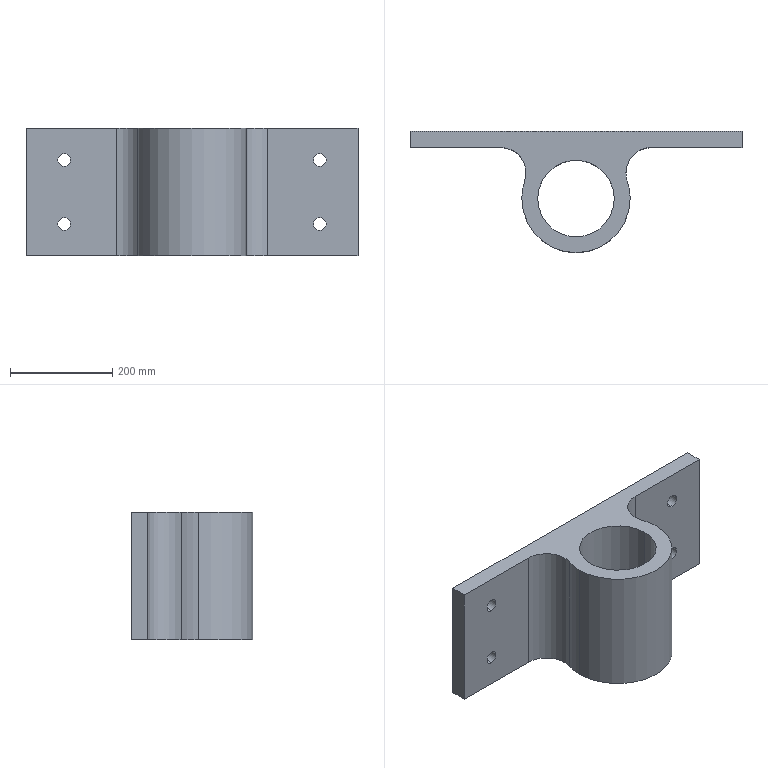Part | SolidWorks | features Extrusion 1, ICE 1 | 1 solid | 23 faces | box 650 x 238 x 250 mm | volume 10403877 mm3 | cylinder 16 | plane 7 | commonest cylinder face diameters 25 x8 100 x3 212 x3 150 x2
STEP:
#1=CARTESIAN_POINT('',(250.,100.,75.));
#2=VERTEX_POINT('',#1);
#3=CARTESIAN_POINT('',(250.,100.,50.));
#4=VERTEX_POINT('',#3);
#5=CARTESIAN_POINT('',(250.,100.,62.5));
#6=DIRECTION('',(0.,-1.,0.));
#7=DIRECTION('',(-1.,0.,0.));
#8=AXIS2_PLACEMENT_3D('',#5,#6,#7);
#9=CIRCLE('',#8,12.5);
#10=EDGE_CURVE('',#2,#4,#9,.T.);
#11=ORIENTED_EDGE('',*,*,#10,.T.);
#12=CARTESIAN_POINT('',(250.,132.,50.));
#13=VERTEX_POINT('',#12);
#14=CARTESIAN_POINT('',(250.,-106.001,50.));
#15=DIRECTION('',(0.,1.,0.));
#16=VECTOR('',#15,1000.);
#17=LINE('',#14,#16);
#18=EDGE_CURVE('',#4,#13,#17,.T.);
#19=ORIENTED_EDGE('',*,*,#18,.T.);
#20=CARTESIAN_POINT('',(250.,132.,75.));
#21=VERTEX_POINT('',#20);
#22=CARTESIAN_POINT('',(250.,132.,62.5));
#23=DIRECTION('',(0.,1.,0.));
#24=DIRECTION('',(0.,0.,1.));
#25=AXIS2_PLACEMENT_3D('',#22,#23,#24);
#26=CIRCLE('',#25,12.5);
#27=EDGE_CURVE('',#13,#21,#26,.T.);
#28=ORIENTED_EDGE('',*,*,#27,.T.);
#29=CARTESIAN_POINT('',(250.,-106.001,75.));
#30=DIRECTION('',(0.,1.,0.));
#31=VECTOR('',#30,1000.);
#32=LINE('',#29,#31);
#33=EDGE_CURVE('',#2,#21,#32,.T.);
#34=ORIENTED_EDGE('',*,*,#33,.F.);
#35=EDGE_LOOP('',(#11,#19,#28,#34));
#36=FACE_OUTER_BOUND('',#35,.T.);
#37=CARTESIAN_POINT('',(250.,-106.001,62.5));
#38=DIRECTION('',(0.,1.,0.));
#39=DIRECTION('',(0.,0.,1.));
#40=AXIS2_PLACEMENT_3D('',#37,#38,#39);
#41=CYLINDRICAL_SURFACE('',#40,12.5);
#42=ADVANCED_FACE('',(#36),#41,.F.);
#43=CARTESIAN_POINT('',(250.,100.,200.));
#44=VERTEX_POINT('',#43);
#45=CARTESIAN_POINT('',(250.,100.,175.));
#46=VERTEX_POINT('',#45);
#47=CARTESIAN_POINT('',(250.,100.,187.5));
#48=DIRECTION('',(0.,-1.,0.));
#49=DIRECTION('',(-1.,0.,0.));
#50=AXIS2_PLACEMENT_3D('',#47,#48,#49);
#51=CIRCLE('',#50,12.5);
#52=EDGE_CURVE('',#44,#46,#51,.T.);
#53=ORIENTED_EDGE('',*,*,#52,.T.);
#54=CARTESIAN_POINT('',(250.,132.,175.));
#55=VERTEX_POINT('',#54);
#56=CARTESIAN_POINT('',(250.,-106.001,175.));
#57=DIRECTION('',(0.,1.,0.));
#58=VECTOR('',#57,1000.);
#59=LINE('',#56,#58);
#60=EDGE_CURVE('',#46,#55,#59,.T.);
#61=ORIENTED_EDGE('',*,*,#60,.T.);
#62=CARTESIAN_POINT('',(250.,132.,200.));
#63=VERTEX_POINT('',#62);
#64=CARTESIAN_POINT('',(250.,132.,187.5));
#65=DIRECTION('',(0.,1.,0.));
#66=DIRECTION('',(0.,0.,1.));
#67=AXIS2_PLACEMENT_3D('',#64,#65,#66);
#68=CIRCLE('',#67,12.5);
#69=EDGE_CURVE('',#55,#63,#68,.T.);
#70=ORIENTED_EDGE('',*,*,#69,.T.);
#71=CARTESIAN_POINT('',(250.,-106.001,200.));
#72=DIRECTION('',(0.,1.,0.));
#73=VECTOR('',#72,1000.);
#74=LINE('',#71,#73);
#75=EDGE_CURVE('',#44,#63,#74,.T.);
#76=ORIENTED_EDGE('',*,*,#75,.F.);
#77=EDGE_LOOP('',(#53,#61,#70,#76));
#78=FACE_OUTER_BOUND('',#77,.T.);
#79=CARTESIAN_POINT('',(250.,-106.001,187.5));
#80=DIRECTION('',(0.,1.,0.));
#81=DIRECTION('',(0.,0.,1.));
#82=AXIS2_PLACEMENT_3D('',#79,#80,#81);
#83=CYLINDRICAL_SURFACE('',#82,12.5);
#84=ADVANCED_FACE('',(#78),#83,.F.);
#85=CARTESIAN_POINT('',(-250.,100.,200.));
#86=VERTEX_POINT('',#85);
#87=CARTESIAN_POINT('',(-250.,100.,175.));
#88=VERTEX_POINT('',#87);
#89=CARTESIAN_POINT('',(-250.,100.,187.5));
#90=DIRECTION('',(0.,-1.,0.));
#91=DIRECTION('',(-1.,0.,0.));
#92=AXIS2_PLACEMENT_3D('',#89,#90,#91);
#93=CIRCLE('',#92,12.5);
#94=EDGE_CURVE('',#86,#88,#93,.T.);
#95=ORIENTED_EDGE('',*,*,#94,.T.);
#96=CARTESIAN_POINT('',(-250.,132.,175.));
#97=VERTEX_POINT('',#96);
#98=CARTESIAN_POINT('',(-250.,-106.001,175.));
#99=DIRECTION('',(0.,1.,0.));
#100=VECTOR('',#99,1000.);
#101=LINE('',#98,#100);
#102=EDGE_CURVE('',#88,#97,#101,.T.);
#103=ORIENTED_EDGE('',*,*,#102,.T.);
#104=CARTESIAN_POINT('',(-250.,132.,200.));
#105=VERTEX_POINT('',#104);
#106=CARTESIAN_POINT('',(-250.,132.,187.5));
#107=DIRECTION('',(0.,1.,0.));
#108=DIRECTION('',(0.,0.,1.));
#109=AXIS2_PLACEMENT_3D('',#106,#107,#108);
#110=CIRCLE('',#109,12.5);
#111=EDGE_CURVE('',#97,#105,#110,.T.);
#112=ORIENTED_EDGE('',*,*,#111,.T.);
#113=CARTESIAN_POINT('',(-250.,-106.001,200.));
#114=DIRECTION('',(0.,1.,0.));
#115=VECTOR('',#114,1000.);
#116=LINE('',#113,#115);
#117=EDGE_CURVE('',#86,#105,#116,.T.);
#118=ORIENTED_EDGE('',*,*,#117,.F.);
#119=EDGE_LOOP('',(#95,#103,#112,#118));
#120=FACE_OUTER_BOUND('',#119,.T.);
#121=CARTESIAN_POINT('',(-250.,-106.001,187.5));
#122=DIRECTION('',(0.,1.,0.));
#123=DIRECTION('',(0.,0.,1.));
#124=AXIS2_PLACEMENT_3D('',#121,#122,#123);
#125=CYLINDRICAL_SURFACE('',#124,12.5);
#126=ADVANCED_FACE('',(#120),#125,.F.);
#127=CARTESIAN_POINT('',(-250.,100.,75.));
#128=VERTEX_POINT('',#127);
#129=CARTESIAN_POINT('',(-250.,100.,50.));
#130=VERTEX_POINT('',#129);
#131=CARTESIAN_POINT('',(-250.,100.,62.5));
#132=DIRECTION('',(0.,-1.,0.));
#133=DIRECTION('',(-1.,0.,0.));
#134=AXIS2_PLACEMENT_3D('',#131,#132,#133);
#135=CIRCLE('',#134,12.5);
#136=EDGE_CURVE('',#128,#130,#135,.T.);
#137=ORIENTED_EDGE('',*,*,#136,.T.);
#138=CARTESIAN_POINT('',(-250.,132.,50.));
#139=VERTEX_POINT('',#138);
#140=CARTESIAN_POINT('',(-250.,-106.001,50.));
#141=DIRECTION('',(0.,1.,0.));
#142=VECTOR('',#141,1000.);
#143=LINE('',#140,#142);
#144=EDGE_CURVE('',#130,#139,#143,.T.);
#145=ORIENTED_EDGE('',*,*,#144,.T.);
#146=CARTESIAN_POINT('',(-250.,132.,75.));
#147=VERTEX_POINT('',#146);
#148=CARTESIAN_POINT('',(-250.,132.,62.5));
#149=DIRECTION('',(0.,1.,0.));
#150=DIRECTION('',(0.,0.,1.));
#151=AXIS2_PLACEMENT_3D('',#148,#149,#150);
#152=CIRCLE('',#151,12.5);
#153=EDGE_CURVE('',#139,#147,#152,.T.);
#154=ORIENTED_EDGE('',*,*,#153,.T.);
#155=CARTESIAN_POINT('',(-250.,-106.001,75.));
#156=DIRECTION('',(0.,1.,0.));
#157=VECTOR('',#156,1000.);
#158=LINE('',#155,#157);
#159=EDGE_CURVE('',#128,#147,#158,.T.);
#160=ORIENTED_EDGE('',*,*,#159,.F.);
#161=EDGE_LOOP('',(#137,#145,#154,#160));
#162=FACE_OUTER_BOUND('',#161,.T.);
#163=CARTESIAN_POINT('',(-250.,-106.001,62.5));
#164=DIRECTION('',(0.,1.,0.));
#165=DIRECTION('',(0.,0.,1.));
#166=AXIS2_PLACEMENT_3D('',#163,#164,#165);
#167=CYLINDRICAL_SURFACE('',#166,12.5);
#168=ADVANCED_FACE('',(#162),#167,.F.);
#169=CARTESIAN_POINT('',(-75.,0.,250.));
#170=VERTEX_POINT('',#169);
#171=CARTESIAN_POINT('',(75.,0.,250.));
#172=VERTEX_POINT('',#171);
#173=CARTESIAN_POINT('',(0.,0.,250.));
#174=DIRECTION('',(0.,0.,1.));
#175=DIRECTION('',(1.,0.,0.));
#176=AXIS2_PLACEMENT_3D('',#173,#174,#175);
#177=CIRCLE('',#176,75.);
#178=EDGE_CURVE('',#170,#172,#177,.T.);
#179=ORIENTED_EDGE('',*,*,#178,.T.);
#180=CARTESIAN_POINT('',(75.,0.,0.));
#181=VERTEX_POINT('',#180);
#182=CARTESIAN_POINT('',(75.,0.,250.));
#183=DIRECTION('',(0.,0.,-1.));
#184=VECTOR('',#183,1000.);
#185=LINE('',#182,#184);
#186=EDGE_CURVE('',#172,#181,#185,.T.);
#187=ORIENTED_EDGE('',*,*,#186,.T.);
#188=CARTESIAN_POINT('',(-75.,0.,0.));
#189=VERTEX_POINT('',#188);
#190=CARTESIAN_POINT('',(0.,0.,0.));
#191=DIRECTION('',(0.,0.,1.));
#192=DIRECTION('',(1.,0.,0.));
#193=AXIS2_PLACEMENT_3D('',#190,#191,#192);
#194=CIRCLE('',#193,75.);
#195=EDGE_CURVE('',#189,#181,#194,.T.);
#196=ORIENTED_EDGE('',*,*,#195,.F.);
#197=CARTESIAN_POINT('',(-75.,0.,250.));
#198=DIRECTION('',(0.,0.,-1.));
#199=VECTOR('',#198,1000.);
#200=LINE('',#197,#199);
#201=EDGE_CURVE('',#170,#189,#200,.T.);
#202=ORIENTED_EDGE('',*,*,#201,.F.);
#203=EDGE_LOOP('',(#179,#187,#196,#202));
#204=FACE_OUTER_BOUND('',#203,.T.);
#205=CARTESIAN_POINT('',(0.,0.,250.));
#206=DIRECTION('',(0.,0.,-1.));
#207=DIRECTION('',(-1.,0.,0.));
#208=AXIS2_PLACEMENT_3D('',#205,#206,#207);
#209=CYLINDRICAL_SURFACE('',#208,75.);
#210=ADVANCED_FACE('',(#204),#209,.F.);
#211=CARTESIAN_POINT('',(97.77,50.,250.));
#212=VERTEX_POINT('',#211);
#213=CARTESIAN_POINT('',(147.77,100.,250.));
#214=VERTEX_POINT('',#213);
#215=CARTESIAN_POINT('',(147.77,50.,250.));
#216=DIRECTION('',(0.,0.,-1.));
#217=DIRECTION('',(-1.,0.,0.));
#218=AXIS2_PLACEMENT_3D('',#215,#216,#217);
#219=CIRCLE('',#218,50.);
#220=EDGE_CURVE('',#212,#214,#219,.T.);
#221=ORIENTED_EDGE('',*,*,#220,.F.);
#222=CARTESIAN_POINT('',(97.77,50.,0.));
#223=VERTEX_POINT('',#222);
#224=CARTESIAN_POINT('',(97.77,50.,250.));
#225=DIRECTION('',(0.,0.,-1.));
#226=VECTOR('',#225,1000.);
#227=LINE('',#224,#226);
#228=EDGE_CURVE('',#212,#223,#227,.T.);
#229=ORIENTED_EDGE('',*,*,#228,.T.);
#230=CARTESIAN_POINT('',(147.77,100.,0.));
#231=VERTEX_POINT('',#230);
#232=CARTESIAN_POINT('',(147.77,50.,0.));
#233=DIRECTION('',(0.,0.,-1.));
#234=DIRECTION('',(-1.,0.,0.));
#235=AXIS2_PLACEMENT_3D('',#232,#233,#234);
#236=CIRCLE('',#235,50.);
#237=EDGE_CURVE('',#223,#231,#236,.T.);
#238=ORIENTED_EDGE('',*,*,#237,.T.);
#239=CARTESIAN_POINT('',(147.77,100.,250.));
#240=DIRECTION('',(0.,0.,-1.));
#241=VECTOR('',#240,1000.);
#242=LINE('',#239,#241);
#243=EDGE_CURVE('',#214,#231,#242,.T.);
#244=ORIENTED_EDGE('',*,*,#243,.F.);
#245=EDGE_LOOP('',(#221,#229,#238,#244));
#246=FACE_OUTER_BOUND('',#245,.T.);
#247=CARTESIAN_POINT('',(147.77,50.,250.));
#248=DIRECTION('',(0.,0.,-1.));
#249=DIRECTION('',(-1.,0.,0.));
#250=AXIS2_PLACEMENT_3D('',#247,#248,#249);
#251=CYLINDRICAL_SURFACE('',#250,50.);
#252=ADVANCED_FACE('',(#246),#251,.F.);
#253=CARTESIAN_POINT('',(106.,0.,250.));
#254=VERTEX_POINT('',#253);
#255=CARTESIAN_POINT('',(100.408,33.974,250.));
#256=VERTEX_POINT('',#255);
#257=CARTESIAN_POINT('',(0.,0.,250.));
#258=DIRECTION('',(0.,0.,1.));
#259=DIRECTION('',(1.,0.,0.));
#260=AXIS2_PLACEMENT_3D('',#257,#258,#259);
#261=CIRCLE('',#260,106.);
#262=EDGE_CURVE('',#254,#256,#261,.T.);
#263=ORIENTED_EDGE('',*,*,#262,.F.);
#264=CARTESIAN_POINT('',(106.,0.,0.));
#265=VERTEX_POINT('',#264);
#266=CARTESIAN_POINT('',(106.,0.,250.));
#267=DIRECTION('',(0.,0.,-1.));
#268=VECTOR('',#267,1000.);
#269=LINE('',#266,#268);
#270=EDGE_CURVE('',#254,#265,#269,.T.);
#271=ORIENTED_EDGE('',*,*,#270,.T.);
#272=CARTESIAN_POINT('',(100.408,33.974,0.));
#273=VERTEX_POINT('',#272);
#274=CARTESIAN_POINT('',(0.,0.,0.));
#275=DIRECTION('',(0.,0.,1.));
#276=DIRECTION('',(1.,0.,0.));
#277=AXIS2_PLACEMENT_3D('',#274,#275,#276);
#278=CIRCLE('',#277,106.);
#279=EDGE_CURVE('',#265,#273,#278,.T.);
#280=ORIENTED_EDGE('',*,*,#279,.T.);
#281=CARTESIAN_POINT('',(100.408,33.974,250.));
#282=DIRECTION('',(0.,0.,-1.));
#283=VECTOR('',#282,1000.);
#284=LINE('',#281,#283);
#285=EDGE_CURVE('',#256,#273,#284,.T.);
#286=ORIENTED_EDGE('',*,*,#285,.F.);
#287=EDGE_LOOP('',(#263,#271,#280,#286));
#288=FACE_OUTER_BOUND('',#287,.T.);
#289=CARTESIAN_POINT('',(0.,0.,250.));
#290=DIRECTION('',(0.,0.,-1.));
#291=DIRECTION('',(-1.,0.,0.));
#292=AXIS2_PLACEMENT_3D('',#289,#290,#291);
#293=CYLINDRICAL_SURFACE('',#292,106.);
#294=ADVANCED_FACE('',(#288),#293,.T.);
#295=ORIENTED_EDGE('',*,*,#270,.F.);
#296=CARTESIAN_POINT('',(-106.,0.,250.));
#297=VERTEX_POINT('',#296);
#298=CARTESIAN_POINT('',(0.,0.,250.));
#299=DIRECTION('',(0.,0.,1.));
#300=DIRECTION('',(1.,0.,0.));
#301=AXIS2_PLACEMENT_3D('',#298,#299,#300);
#302=CIRCLE('',#301,106.);
#303=EDGE_CURVE('',#297,#254,#302,.T.);
#304=ORIENTED_EDGE('',*,*,#303,.F.);
#305=CARTESIAN_POINT('',(-106.,0.,0.));
#306=VERTEX_POINT('',#305);
#307=CARTESIAN_POINT('',(-106.,0.,250.));
#308=DIRECTION('',(0.,0.,-1.));
#309=VECTOR('',#308,1000.);
#310=LINE('',#307,#309);
#311=EDGE_CURVE('',#297,#306,#310,.T.);
#312=ORIENTED_EDGE('',*,*,#311,.T.);
#313=CARTESIAN_POINT('',(0.,0.,0.));
#314=DIRECTION('',(0.,0.,1.));
#315=DIRECTION('',(1.,0.,0.));
#316=AXIS2_PLACEMENT_3D('',#313,#314,#315);
#317=CIRCLE('',#316,106.);
#318=EDGE_CURVE('',#306,#265,#317,.T.);
#319=ORIENTED_EDGE('',*,*,#318,.T.);
#320=EDGE_LOOP('',(#295,#304,#312,#319));
#321=FACE_OUTER_BOUND('',#320,.T.);
#322=CARTESIAN_POINT('',(0.,0.,250.));
#323=DIRECTION('',(0.,0.,-1.));
#324=DIRECTION('',(-1.,0.,0.));
#325=AXIS2_PLACEMENT_3D('',#322,#323,#324);
#326=CYLINDRICAL_SURFACE('',#325,106.);
#327=ADVANCED_FACE('',(#321),#326,.T.);
#328=CARTESIAN_POINT('',(325.,100.,250.));
#329=VERTEX_POINT('',#328);
#330=CARTESIAN_POINT('',(325.,132.,250.));
#331=VERTEX_POINT('',#330);
#332=CARTESIAN_POINT('',(325.,132.,250.));
#333=DIRECTION('',(0.,1.,0.));
#334=VECTOR('',#333,1000.);
#335=LINE('',#332,#334);
#336=EDGE_CURVE('',#329,#331,#335,.T.);
#337=ORIENTED_EDGE('',*,*,#336,.T.);
#338=CARTESIAN_POINT('',(-325.,132.,250.));
#339=VERTEX_POINT('',#338);
#340=CARTESIAN_POINT('',(325.,132.,250.));
#341=DIRECTION('',(-1.,0.,0.));
#342=VECTOR('',#341,1000.);
#343=LINE('',#340,#342);
#344=EDGE_CURVE('',#331,#339,#343,.T.);
#345=ORIENTED_EDGE('',*,*,#344,.T.);
#346=CARTESIAN_POINT('',(-325.,100.,250.));
#347=VERTEX_POINT('',#346);
#348=CARTESIAN_POINT('',(-325.,132.,250.));
#349=DIRECTION('',(0.,-1.,0.));
#350=VECTOR('',#349,1000.);
#351=LINE('',#348,#350);
#352=EDGE_CURVE('',#339,#347,#351,.T.);
#353=ORIENTED_EDGE('',*,*,#352,.T.);
#354=CARTESIAN_POINT('',(-147.77,100.,250.));
#355=VERTEX_POINT('',#354);
#356=CARTESIAN_POINT('',(-325.,100.,250.));
#357=DIRECTION('',(1.,0.,0.));
#358=VECTOR('',#357,1000.);
#359=LINE('',#356,#358);
#360=EDGE_CURVE('',#347,#355,#359,.T.);
#361=ORIENTED_EDGE('',*,*,#360,.T.);
#362=CARTESIAN_POINT('',(-100.408,33.974,250.));
#363=VERTEX_POINT('',#362);
#364=CARTESIAN_POINT('',(-147.77,50.,250.));
#365=DIRECTION('',(0.,0.,-1.));
#366=DIRECTION('',(1.,0.,0.));
#367=AXIS2_PLACEMENT_3D('',#364,#365,#366);
#368=CIRCLE('',#367,50.);
#369=EDGE_CURVE('',#355,#363,#368,.T.);
#370=ORIENTED_EDGE('',*,*,#369,.T.);
#371=CARTESIAN_POINT('',(0.,0.,250.));
#372=DIRECTION('',(0.,0.,1.));
#373=DIRECTION('',(1.,0.,0.));
#374=AXIS2_PLACEMENT_3D('',#371,#372,#373);
#375=CIRCLE('',#374,106.);
#376=EDGE_CURVE('',#363,#297,#375,.T.);
#377=ORIENTED_EDGE('',*,*,#376,.T.);
#378=ORIENTED_EDGE('',*,*,#303,.T.);
#379=ORIENTED_EDGE('',*,*,#262,.T.);
#380=CARTESIAN_POINT('',(147.77,50.,250.));
#381=DIRECTION('',(0.,0.,-1.));
#382=DIRECTION('',(-1.,0.,0.));
#383=AXIS2_PLACEMENT_3D('',#380,#381,#382);
#384=CIRCLE('',#383,50.);
#385=EDGE_CURVE('',#256,#212,#384,.T.);
#386=ORIENTED_EDGE('',*,*,#385,.T.);
#387=ORIENTED_EDGE('',*,*,#220,.T.);
#388=CARTESIAN_POINT('',(325.,100.,250.));
#389=DIRECTION('',(1.,0.,0.));
#390=VECTOR('',#389,1000.);
#391=LINE('',#388,#390);
#392=EDGE_CURVE('',#214,#329,#391,.T.);
#393=ORIENTED_EDGE('',*,*,#392,.T.);
#394=EDGE_LOOP('',(#337,#345,#353,#361,#370,#377,#378,#379,#386,#387,#393));
#395=FACE_OUTER_BOUND('',#394,.T.);
#396=ORIENTED_EDGE('',*,*,#178,.F.);
#397=CARTESIAN_POINT('',(0.,0.,250.));
#398=DIRECTION('',(0.,0.,1.));
#399=DIRECTION('',(1.,0.,0.));
#400=AXIS2_PLACEMENT_3D('',#397,#398,#399);
#401=CIRCLE('',#400,75.);
#402=EDGE_CURVE('',#172,#170,#401,.T.);
#403=ORIENTED_EDGE('',*,*,#402,.F.);
#404=EDGE_LOOP('',(#396,#403));
#405=FACE_BOUND('',#404,.T.);
#406=CARTESIAN_POINT('',(147.77,50.,250.));
#407=DIRECTION('',(0.,0.,-1.));
#408=DIRECTION('',(-1.,0.,0.));
#409=AXIS2_PLACEMENT_3D('',#406,#407,#408);
#410=PLANE('',#409);
#411=ADVANCED_FACE('',(#395,#405),#410,.F.);
#412=CARTESIAN_POINT('',(325.,100.,0.));
#413=VERTEX_POINT('',#412);
#414=CARTESIAN_POINT('',(325.,132.,0.));
#415=VERTEX_POINT('',#414);
#416=CARTESIAN_POINT('',(325.,132.,0.));
#417=DIRECTION('',(0.,1.,0.));
#418=VECTOR('',#417,1000.);
#419=LINE('',#416,#418);
#420=EDGE_CURVE('',#413,#415,#419,.T.);
#421=ORIENTED_EDGE('',*,*,#420,.F.);
#422=CARTESIAN_POINT('',(325.,100.,0.));
#423=DIRECTION('',(1.,0.,0.));
#424=VECTOR('',#423,1000.);
#425=LINE('',#422,#424);
#426=EDGE_CURVE('',#231,#413,#425,.T.);
#427=ORIENTED_EDGE('',*,*,#426,.F.);
#428=ORIENTED_EDGE('',*,*,#237,.F.);
#429=CARTESIAN_POINT('',(147.77,50.,0.));
#430=DIRECTION('',(0.,0.,-1.));
#431=DIRECTION('',(-1.,0.,0.));
#432=AXIS2_PLACEMENT_3D('',#429,#430,#431);
#433=CIRCLE('',#432,50.);
#434=EDGE_CURVE('',#273,#223,#433,.T.);
#435=ORIENTED_EDGE('',*,*,#434,.F.);
#436=ORIENTED_EDGE('',*,*,#279,.F.);
#437=ORIENTED_EDGE('',*,*,#318,.F.);
#438=CARTESIAN_POINT('',(-100.408,33.974,0.));
#439=VERTEX_POINT('',#438);
#440=CARTESIAN_POINT('',(0.,0.,0.));
#441=DIRECTION('',(0.,0.,1.));
#442=DIRECTION('',(1.,0.,0.));
#443=AXIS2_PLACEMENT_3D('',#440,#441,#442);
#444=CIRCLE('',#443,106.);
#445=EDGE_CURVE('',#439,#306,#444,.T.);
#446=ORIENTED_EDGE('',*,*,#445,.F.);
#447=CARTESIAN_POINT('',(-147.77,100.,0.));
#448=VERTEX_POINT('',#447);
#449=CARTESIAN_POINT('',(-147.77,50.,0.));
#450=DIRECTION('',(0.,0.,-1.));
#451=DIRECTION('',(1.,0.,0.));
#452=AXIS2_PLACEMENT_3D('',#449,#450,#451);
#453=CIRCLE('',#452,50.);
#454=EDGE_CURVE('',#448,#439,#453,.T.);
#455=ORIENTED_EDGE('',*,*,#454,.F.);
#456=CARTESIAN_POINT('',(-325.,100.,0.));
#457=VERTEX_POINT('',#456);
#458=CARTESIAN_POINT('',(-325.,100.,0.));
#459=DIRECTION('',(1.,0.,0.));
#460=VECTOR('',#459,1000.);
#461=LINE('',#458,#460);
#462=EDGE_CURVE('',#457,#448,#461,.T.);
#463=ORIENTED_EDGE('',*,*,#462,.F.);
#464=CARTESIAN_POINT('',(-325.,132.,0.));
#465=VERTEX_POINT('',#464);
#466=CARTESIAN_POINT('',(-325.,132.,0.));
#467=DIRECTION('',(0.,-1.,0.));
#468=VECTOR('',#467,1000.);
#469=LINE('',#466,#468);
#470=EDGE_CURVE('',#465,#457,#469,.T.);
#471=ORIENTED_EDGE('',*,*,#470,.F.);
#472=CARTESIAN_POINT('',(325.,132.,0.));
#473=DIRECTION('',(-1.,0.,0.));
#474=VECTOR('',#473,1000.);
#475=LINE('',#472,#474);
#476=EDGE_CURVE('',#415,#465,#475,.T.);
#477=ORIENTED_EDGE('',*,*,#476,.F.);
#478=EDGE_LOOP('',(#421,#427,#428,#435,#436,#437,#446,#455,#463,#471,#477));
#479=FACE_OUTER_BOUND('',#478,.T.);
#480=ORIENTED_EDGE('',*,*,#195,.T.);
#481=CARTESIAN_POINT('',(0.,0.,0.));
#482=DIRECTION('',(0.,0.,1.));
#483=DIRECTION('',(1.,0.,0.));
#484=AXIS2_PLACEMENT_3D('',#481,#482,#483);
#485=CIRCLE('',#484,75.);
#486=EDGE_CURVE('',#181,#189,#485,.T.);
#487=ORIENTED_EDGE('',*,*,#486,.T.);
#488=EDGE_LOOP('',(#480,#487));
#489=FACE_BOUND('',#488,.T.);
#490=CARTESIAN_POINT('',(147.77,50.,0.));
#491=DIRECTION('',(0.,0.,-1.));
#492=DIRECTION('',(-1.,0.,0.));
#493=AXIS2_PLACEMENT_3D('',#490,#491,#492);
#494=PLANE('',#493);
#495=ADVANCED_FACE('',(#479,#489),#494,.T.);
#496=ORIENTED_EDGE('',*,*,#420,.T.);
#497=CARTESIAN_POINT('',(325.,132.,250.));
#498=DIRECTION('',(0.,0.,-1.));
#499=VECTOR('',#498,1000.);
#500=LINE('',#497,#499);
#501=EDGE_CURVE('',#331,#415,#500,.T.);
#502=ORIENTED_EDGE('',*,*,#501,.F.);
#503=ORIENTED_EDGE('',*,*,#336,.F.);
#504=CARTESIAN_POINT('',(325.,100.,250.));
#505=DIRECTION('',(0.,0.,-1.));
#506=VECTOR('',#505,1000.);
#507=LINE('',#504,#506);
#508=EDGE_CURVE('',#329,#413,#507,.T.);
#509=ORIENTED_EDGE('',*,*,#508,.T.);
#510=EDGE_LOOP('',(#496,#502,#503,#509));
#511=FACE_OUTER_BOUND('',#510,.T.);
#512=CARTESIAN_POINT('',(325.,132.,250.));
#513=DIRECTION('',(-1.,0.,0.));
#514=DIRECTION('',(0.,-1.,0.));
#515=AXIS2_PLACEMENT_3D('',#512,#513,#514);
#516=PLANE('',#515);
#517=ADVANCED_FACE('',(#511),#516,.F.);
#518=CARTESIAN_POINT('',(250.,132.,62.5));
#519=DIRECTION('',(0.,1.,0.));
#520=DIRECTION('',(0.,0.,1.));
#521=AXIS2_PLACEMENT_3D('',#518,#519,#520);
#522=CIRCLE('',#521,12.5);
#523=EDGE_CURVE('',#21,#13,#522,.T.);
#524=ORIENTED_EDGE('',*,*,#523,.F.);
#525=ORIENTED_EDGE('',*,*,#27,.F.);
#526=EDGE_LOOP('',(#524,#525));
#527=FACE_BOUND('',#526,.T.);
#528=CARTESIAN_POINT('',(250.,132.,187.5));
#529=DIRECTION('',(0.,1.,0.));
#530=DIRECTION('',(0.,0.,1.));
#531=AXIS2_PLACEMENT_3D('',#528,#529,#530);
#532=CIRCLE('',#531,12.5);
#533=EDGE_CURVE('',#63,#55,#532,.T.);
#534=ORIENTED_EDGE('',*,*,#533,.F.);
#535=ORIENTED_EDGE('',*,*,#69,.F.);
#536=EDGE_LOOP('',(#534,#535));
#537=FACE_BOUND('',#536,.T.);
#538=CARTESIAN_POINT('',(-250.,132.,187.5));
#539=DIRECTION('',(0.,1.,0.));
#540=DIRECTION('',(0.,0.,1.));
#541=AXIS2_PLACEMENT_3D('',#538,#539,#540);
#542=CIRCLE('',#541,12.5);
#543=EDGE_CURVE('',#105,#97,#542,.T.);
#544=ORIENTED_EDGE('',*,*,#543,.F.);
#545=ORIENTED_EDGE('',*,*,#111,.F.);
#546=EDGE_LOOP('',(#544,#545));
#547=FACE_BOUND('',#546,.T.);
#548=CARTESIAN_POINT('',(-250.,132.,62.5));
#549=DIRECTION('',(0.,1.,0.));
#550=DIRECTION('',(0.,0.,1.));
#551=AXIS2_PLACEMENT_3D('',#548,#549,#550);
#552=CIRCLE('',#551,12.5);
#553=EDGE_CURVE('',#147,#139,#552,.T.);
#554=ORIENTED_EDGE('',*,*,#553,.F.);
#555=ORIENTED_EDGE('',*,*,#153,.F.);
#556=EDGE_LOOP('',(#554,#555));
#557=FACE_BOUND('',#556,.T.);
#558=ORIENTED_EDGE('',*,*,#476,.T.);
#559=CARTESIAN_POINT('',(-325.,132.,250.));
#560=DIRECTION('',(0.,0.,-1.));
#561=VECTOR('',#560,1000.);
#562=LINE('',#559,#561);
#563=EDGE_CURVE('',#339,#465,#562,.T.);
#564=ORIENTED_EDGE('',*,*,#563,.F.);
#565=ORIENTED_EDGE('',*,*,#344,.F.);
#566=ORIENTED_EDGE('',*,*,#501,.T.);
#567=EDGE_LOOP('',(#558,#564,#565,#566));
#568=FACE_OUTER_BOUND('',#567,.T.);
#569=CARTESIAN_POINT('',(325.,132.,250.));
#570=DIRECTION('',(0.,-1.,0.));
#571=DIRECTION('',(0.,0.,-1.));
#572=AXIS2_PLACEMENT_3D('',#569,#570,#571);
#573=PLANE('',#572);
#574=ADVANCED_FACE('',(#527,#537,#547,#557,#568),#573,.F.);
#575=ORIENTED_EDGE('',*,*,#470,.T.);
#576=CARTESIAN_POINT('',(-325.,100.,250.));
#577=DIRECTION('',(0.,0.,-1.));
#578=VECTOR('',#577,1000.);
#579=LINE('',#576,#578);
#580=EDGE_CURVE('',#347,#457,#579,.T.);
#581=ORIENTED_EDGE('',*,*,#580,.F.);
#582=ORIENTED_EDGE('',*,*,#352,.F.);
#583=ORIENTED_EDGE('',*,*,#563,.T.);
#584=EDGE_LOOP('',(#575,#581,#582,#583));
#585=FACE_OUTER_BOUND('',#584,.T.);
#586=CARTESIAN_POINT('',(-325.,132.,250.));
#587=DIRECTION('',(1.,0.,0.));
#588=DIRECTION('',(0.,1.,0.));
#589=AXIS2_PLACEMENT_3D('',#586,#587,#588);
#590=PLANE('',#589);
#591=ADVANCED_FACE('',(#585),#590,.F.);
#592=ORIENTED_EDGE('',*,*,#94,.F.);
#593=CARTESIAN_POINT('',(-250.,100.,187.5));
#594=DIRECTION('',(0.,-1.,0.));
#595=DIRECTION('',(-1.,0.,0.));
#596=AXIS2_PLACEMENT_3D('',#593,#594,#595);
#597=CIRCLE('',#596,12.5);
#598=EDGE_CURVE('',#88,#86,#597,.T.);
#599=ORIENTED_EDGE('',*,*,#598,.F.);
#600=EDGE_LOOP('',(#592,#599));
#601=FACE_BOUND('',#600,.T.);
#602=ORIENTED_EDGE('',*,*,#136,.F.);
#603=CARTESIAN_POINT('',(-250.,100.,62.5));
#604=DIRECTION('',(0.,-1.,0.));
#605=DIRECTION('',(-1.,0.,0.));
#606=AXIS2_PLACEMENT_3D('',#603,#604,#605);
#607=CIRCLE('',#606,12.5);
#608=EDGE_CURVE('',#130,#128,#607,.T.);
#609=ORIENTED_EDGE('',*,*,#608,.F.);
#610=EDGE_LOOP('',(#602,#609));
#611=FACE_BOUND('',#610,.T.);
#612=ORIENTED_EDGE('',*,*,#462,.T.);
#613=CARTESIAN_POINT('',(-147.77,100.,250.));
#614=DIRECTION('',(0.,0.,-1.));
#615=VECTOR('',#614,1000.);
#616=LINE('',#613,#615);
#617=EDGE_CURVE('',#355,#448,#616,.T.);
#618=ORIENTED_EDGE('',*,*,#617,.F.);
#619=ORIENTED_EDGE('',*,*,#360,.F.);
#620=ORIENTED_EDGE('',*,*,#580,.T.);
#621=EDGE_LOOP('',(#612,#618,#619,#620));
#622=FACE_OUTER_BOUND('',#621,.T.);
#623=CARTESIAN_POINT('',(-325.,100.,250.));
#624=DIRECTION('',(0.,1.,0.));
#625=DIRECTION('',(-1.,0.,0.));
#626=AXIS2_PLACEMENT_3D('',#623,#624,#625);
#627=PLANE('',#626);
#628=ADVANCED_FACE('',(#601,#611,#622),#627,.F.);
#629=ORIENTED_EDGE('',*,*,#454,.T.);
#630=CARTESIAN_POINT('',(-100.408,33.974,250.));
#631=DIRECTION('',(0.,0.,-1.));
#632=VECTOR('',#631,1000.);
#633=LINE('',#630,#632);
#634=EDGE_CURVE('',#363,#439,#633,.T.);
#635=ORIENTED_EDGE('',*,*,#634,.F.);
#636=ORIENTED_EDGE('',*,*,#369,.F.);
#637=ORIENTED_EDGE('',*,*,#617,.T.);
#638=EDGE_LOOP('',(#629,#635,#636,#637));
#639=FACE_OUTER_BOUND('',#638,.T.);
#640=CARTESIAN_POINT('',(-147.77,50.,250.));
#641=DIRECTION('',(0.,0.,-1.));
#642=DIRECTION('',(-1.,0.,0.));
#643=AXIS2_PLACEMENT_3D('',#640,#641,#642);
#644=CYLINDRICAL_SURFACE('',#643,50.);
#645=ADVANCED_FACE('',(#639),#644,.F.);
#646=ORIENTED_EDGE('',*,*,#311,.F.);
#647=ORIENTED_EDGE('',*,*,#376,.F.);
#648=ORIENTED_EDGE('',*,*,#634,.T.);
#649=ORIENTED_EDGE('',*,*,#445,.T.);
#650=EDGE_LOOP('',(#646,#647,#648,#649));
#651=FACE_OUTER_BOUND('',#650,.T.);
#652=CARTESIAN_POINT('',(0.,0.,250.));
#653=DIRECTION('',(0.,0.,-1.));
#654=DIRECTION('',(-1.,0.,0.));
#655=AXIS2_PLACEMENT_3D('',#652,#653,#654);
#656=CYLINDRICAL_SURFACE('',#655,106.);
#657=ADVANCED_FACE('',(#651),#656,.T.);
#658=ORIENTED_EDGE('',*,*,#228,.F.);
#659=ORIENTED_EDGE('',*,*,#385,.F.);
#660=ORIENTED_EDGE('',*,*,#285,.T.);
#661=ORIENTED_EDGE('',*,*,#434,.T.);
#662=EDGE_LOOP('',(#658,#659,#660,#661));
#663=FACE_OUTER_BOUND('',#662,.T.);
#664=CARTESIAN_POINT('',(147.77,50.,250.));
#665=DIRECTION('',(0.,0.,-1.));
#666=DIRECTION('',(-1.,0.,0.));
#667=AXIS2_PLACEMENT_3D('',#664,#665,#666);
#668=CYLINDRICAL_SURFACE('',#667,50.);
#669=ADVANCED_FACE('',(#663),#668,.F.);
#670=ORIENTED_EDGE('',*,*,#10,.F.);
#671=CARTESIAN_POINT('',(250.,100.,62.5));
#672=DIRECTION('',(0.,-1.,0.));
#673=DIRECTION('',(-1.,0.,0.));
#674=AXIS2_PLACEMENT_3D('',#671,#672,#673);
#675=CIRCLE('',#674,12.5);
#676=EDGE_CURVE('',#4,#2,#675,.T.);
#677=ORIENTED_EDGE('',*,*,#676,.F.);
#678=EDGE_LOOP('',(#670,#677));
#679=FACE_BOUND('',#678,.T.);
#680=ORIENTED_EDGE('',*,*,#52,.F.);
#681=CARTESIAN_POINT('',(250.,100.,187.5));
#682=DIRECTION('',(0.,-1.,0.));
#683=DIRECTION('',(-1.,0.,0.));
#684=AXIS2_PLACEMENT_3D('',#681,#682,#683);
#685=CIRCLE('',#684,12.5);
#686=EDGE_CURVE('',#46,#44,#685,.T.);
#687=ORIENTED_EDGE('',*,*,#686,.F.);
#688=EDGE_LOOP('',(#680,#687));
#689=FACE_BOUND('',#688,.T.);
#690=ORIENTED_EDGE('',*,*,#426,.T.);
#691=ORIENTED_EDGE('',*,*,#508,.F.);
#692=ORIENTED_EDGE('',*,*,#392,.F.);
#693=ORIENTED_EDGE('',*,*,#243,.T.);
#694=EDGE_LOOP('',(#690,#691,#692,#693));
#695=FACE_OUTER_BOUND('',#694,.T.);
#696=CARTESIAN_POINT('',(325.,100.,250.));
#697=DIRECTION('',(0.,1.,0.));
#698=DIRECTION('',(-1.,0.,0.));
#699=AXIS2_PLACEMENT_3D('',#696,#697,#698);
#700=PLANE('',#699);
#701=ADVANCED_FACE('',(#679,#689,#695),#700,.F.);
#702=ORIENTED_EDGE('',*,*,#186,.F.);
#703=ORIENTED_EDGE('',*,*,#402,.T.);
#704=ORIENTED_EDGE('',*,*,#201,.T.);
#705=ORIENTED_EDGE('',*,*,#486,.F.);
#706=EDGE_LOOP('',(#702,#703,#704,#705));
#707=FACE_OUTER_BOUND('',#706,.T.);
#708=CARTESIAN_POINT('',(0.,0.,250.));
#709=DIRECTION('',(0.,0.,-1.));
#710=DIRECTION('',(-1.,0.,0.));
#711=AXIS2_PLACEMENT_3D('',#708,#709,#710);
#712=CYLINDRICAL_SURFACE('',#711,75.);
#713=ADVANCED_FACE('',(#707),#712,.F.);
#714=ORIENTED_EDGE('',*,*,#144,.F.);
#715=ORIENTED_EDGE('',*,*,#608,.T.);
#716=ORIENTED_EDGE('',*,*,#159,.T.);
#717=ORIENTED_EDGE('',*,*,#553,.T.);
#718=EDGE_LOOP('',(#714,#715,#716,#717));
#719=FACE_OUTER_BOUND('',#718,.T.);
#720=CARTESIAN_POINT('',(-250.,-106.001,62.5));
#721=DIRECTION('',(0.,1.,0.));
#722=DIRECTION('',(0.,0.,1.));
#723=AXIS2_PLACEMENT_3D('',#720,#721,#722);
#724=CYLINDRICAL_SURFACE('',#723,12.5);
#725=ADVANCED_FACE('',(#719),#724,.F.);
#726=ORIENTED_EDGE('',*,*,#102,.F.);
#727=ORIENTED_EDGE('',*,*,#598,.T.);
#728=ORIENTED_EDGE('',*,*,#117,.T.);
#729=ORIENTED_EDGE('',*,*,#543,.T.);
#730=EDGE_LOOP('',(#726,#727,#728,#729));
#731=FACE_OUTER_BOUND('',#730,.T.);
#732=CARTESIAN_POINT('',(-250.,-106.001,187.5));
#733=DIRECTION('',(0.,1.,0.));
#734=DIRECTION('',(0.,0.,1.));
#735=AXIS2_PLACEMENT_3D('',#732,#733,#734);
#736=CYLINDRICAL_SURFACE('',#735,12.5);
#737=ADVANCED_FACE('',(#731),#736,.F.);
#738=ORIENTED_EDGE('',*,*,#60,.F.);
#739=ORIENTED_EDGE('',*,*,#686,.T.);
#740=ORIENTED_EDGE('',*,*,#75,.T.);
#741=ORIENTED_EDGE('',*,*,#533,.T.);
#742=EDGE_LOOP('',(#738,#739,#740,#741));
#743=FACE_OUTER_BOUND('',#742,.T.);
#744=CARTESIAN_POINT('',(250.,-106.001,187.5));
#745=DIRECTION('',(0.,1.,0.));
#746=DIRECTION('',(0.,0.,1.));
#747=AXIS2_PLACEMENT_3D('',#744,#745,#746);
#748=CYLINDRICAL_SURFACE('',#747,12.5);
#749=ADVANCED_FACE('',(#743),#748,.F.);
#750=ORIENTED_EDGE('',*,*,#18,.F.);
#751=ORIENTED_EDGE('',*,*,#676,.T.);
#752=ORIENTED_EDGE('',*,*,#33,.T.);
#753=ORIENTED_EDGE('',*,*,#523,.T.);
#754=EDGE_LOOP('',(#750,#751,#752,#753));
#755=FACE_OUTER_BOUND('',#754,.T.);
#756=CARTESIAN_POINT('',(250.,-106.001,62.5));
#757=DIRECTION('',(0.,1.,0.));
#758=DIRECTION('',(0.,0.,1.));
#759=AXIS2_PLACEMENT_3D('',#756,#757,#758);
#760=CYLINDRICAL_SURFACE('',#759,12.5);
#761=ADVANCED_FACE('',(#755),#760,.F.);
#762=CLOSED_SHELL('',(#42,#84,#126,#168,#210,#252,#294,#327,#411,#495,#517,#574,#591,#628,#645,#657,#669,#701,#713,#725,#737,#749,#761));
#763=MANIFOLD_SOLID_BREP('',#762);
#764=CARTESIAN_POINT('',(0.,0.,0.));
#765=DIRECTION('',(0.,0.,1.));
#766=DIRECTION('',(1.,0.,0.));
#767=AXIS2_PLACEMENT_3D('',#764,#765,#766);
#768=(LENGTH_UNIT()NAMED_UNIT(*)SI_UNIT(.MILLI.,.METRE.));
#769=UNCERTAINTY_MEASURE_WITH_UNIT(LENGTH_MEASURE(0.00001),#768,'','');
#770=(NAMED_UNIT(*)PLANE_ANGLE_UNIT()SI_UNIT($,.RADIAN.));
#771=(NAMED_UNIT(*)SI_UNIT($,.STERADIAN.)SOLID_ANGLE_UNIT());
#772=(GEOMETRIC_REPRESENTATION_CONTEXT(3)GLOBAL_UNCERTAINTY_ASSIGNED_CONTEXT((#769))GLOBAL_UNIT_ASSIGNED_CONTEXT((#768,#770,#771))REPRESENTATION_CONTEXT('',''));
#773=ADVANCED_BREP_SHAPE_REPRESENTATION('',(#763,#767),#772);